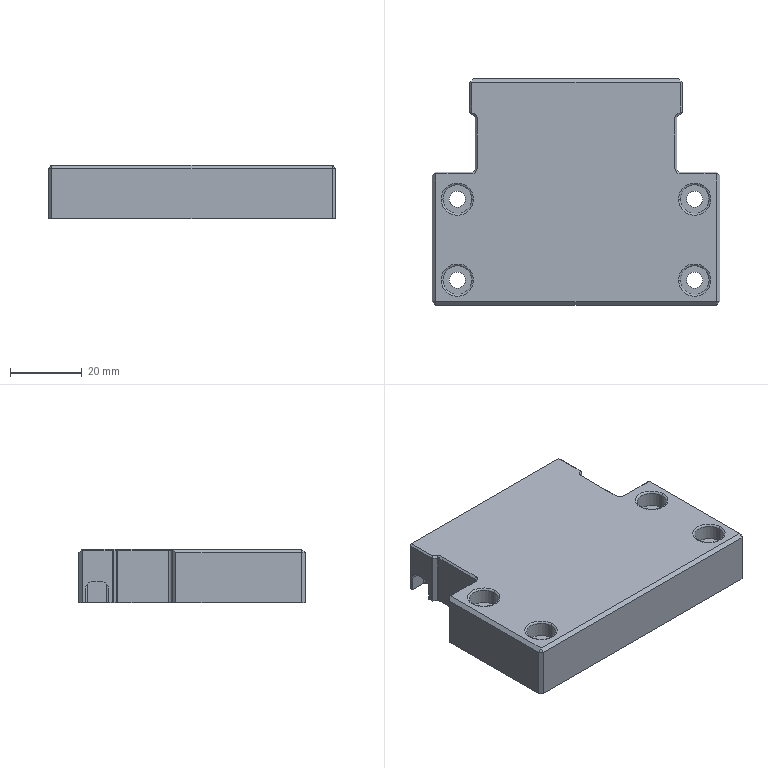Part | NX | features BREP 1 | 1 solid | 94 faces | box 80 x 63 x 15 mm | volume 64331 mm3 | plane 50 | cylinder 30 | torus 8 | cone 6 | commonest cylinder face diameters 1 x8 4.5 x8 8 x8 4 x4 2 x2